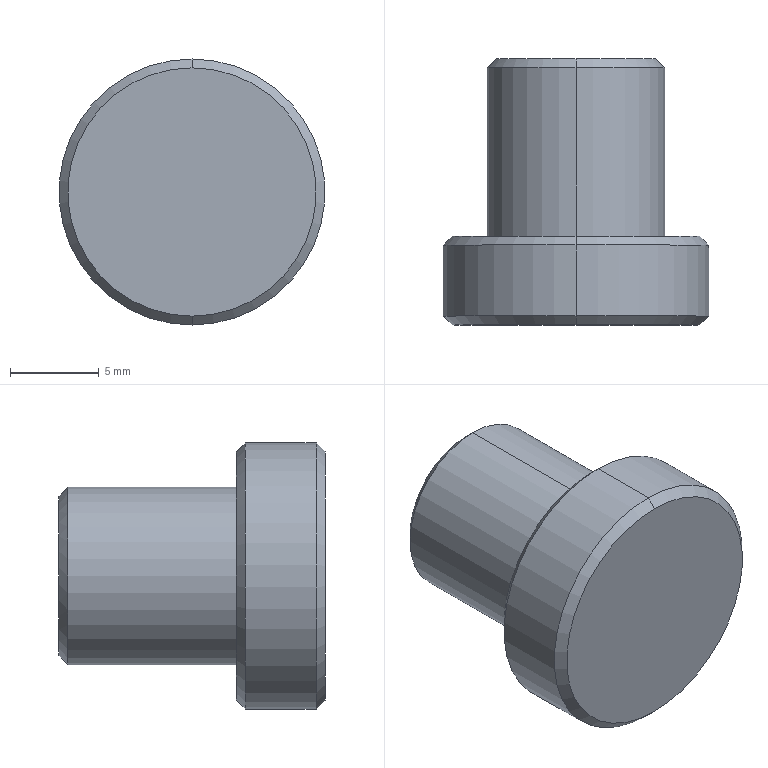Part | SolidWorks | features Chamfer 1, Revolution 1 | 1 solid | 13 faces | box 15 x 15 x 15 mm | volume 1654 mm3 | cone 6 | cylinder 4 | plane 3 | commonest cylinder face diameters 10 x2 15 x2
STEP:
#1=CARTESIAN_POINT('',(0.,15.,4.5));
#2=VERTEX_POINT('',#1);
#3=CARTESIAN_POINT('',(0.,15.,-4.5));
#4=VERTEX_POINT('',#3);
#5=CARTESIAN_POINT('',(0.,15.,0.));
#6=DIRECTION('',(0.,1.,0.));
#7=DIRECTION('',(0.,0.,1.));
#8=AXIS2_PLACEMENT_3D('',#5,#6,#7);
#9=CIRCLE('',#8,4.5);
#10=EDGE_CURVE('',#2,#4,#9,.T.);
#11=ORIENTED_EDGE('',*,*,#10,.F.);
#12=CARTESIAN_POINT('',(0.,14.5,5.));
#13=VERTEX_POINT('',#12);
#14=CARTESIAN_POINT('',(0.,14.5,5.));
#15=DIRECTION('',(0.,-0.7071,0.7071));
#16=VECTOR('',#15,1000.);
#17=LINE('',#14,#16);
#18=EDGE_CURVE('',#2,#13,#17,.T.);
#19=ORIENTED_EDGE('',*,*,#18,.T.);
#20=CARTESIAN_POINT('',(0.,14.5,-5.));
#21=VERTEX_POINT('',#20);
#22=CARTESIAN_POINT('',(0.,14.5,0.));
#23=DIRECTION('',(0.,-1.,0.));
#24=DIRECTION('',(0.,0.,1.));
#25=AXIS2_PLACEMENT_3D('',#22,#23,#24);
#26=CIRCLE('',#25,5.);
#27=EDGE_CURVE('',#21,#13,#26,.T.);
#28=ORIENTED_EDGE('',*,*,#27,.F.);
#29=CARTESIAN_POINT('',(0.,14.5,-5.));
#30=DIRECTION('',(0.,-0.7071,-0.7071));
#31=VECTOR('',#30,1000.);
#32=LINE('',#29,#31);
#33=EDGE_CURVE('',#4,#21,#32,.T.);
#34=ORIENTED_EDGE('',*,*,#33,.F.);
#35=EDGE_LOOP('',(#11,#19,#28,#34));
#36=FACE_OUTER_BOUND('',#35,.T.);
#37=CARTESIAN_POINT('',(0.,14.5,0.));
#38=DIRECTION('',(0.,-1.,0.));
#39=DIRECTION('',(0.,0.,-1.));
#40=AXIS2_PLACEMENT_3D('',#37,#38,#39);
#41=CONICAL_SURFACE('',#40,5.,0.7854);
#42=ADVANCED_FACE('',(#36),#41,.T.);
#43=CARTESIAN_POINT('',(0.,5.,7.));
#44=VERTEX_POINT('',#43);
#45=CARTESIAN_POINT('',(0.,5.,-7.));
#46=VERTEX_POINT('',#45);
#47=CARTESIAN_POINT('',(0.,5.,0.));
#48=DIRECTION('',(0.,1.,0.));
#49=DIRECTION('',(0.,0.,1.));
#50=AXIS2_PLACEMENT_3D('',#47,#48,#49);
#51=CIRCLE('',#50,7.);
#52=EDGE_CURVE('',#44,#46,#51,.T.);
#53=ORIENTED_EDGE('',*,*,#52,.F.);
#54=CARTESIAN_POINT('',(0.,4.5,7.5));
#55=VERTEX_POINT('',#54);
#56=CARTESIAN_POINT('',(0.,4.5,7.5));
#57=DIRECTION('',(0.,-0.7071,0.7071));
#58=VECTOR('',#57,1000.);
#59=LINE('',#56,#58);
#60=EDGE_CURVE('',#44,#55,#59,.T.);
#61=ORIENTED_EDGE('',*,*,#60,.T.);
#62=CARTESIAN_POINT('',(0.,4.5,-7.5));
#63=VERTEX_POINT('',#62);
#64=CARTESIAN_POINT('',(0.,4.5,0.));
#65=DIRECTION('',(0.,-1.,0.));
#66=DIRECTION('',(0.,0.,1.));
#67=AXIS2_PLACEMENT_3D('',#64,#65,#66);
#68=CIRCLE('',#67,7.5);
#69=EDGE_CURVE('',#63,#55,#68,.T.);
#70=ORIENTED_EDGE('',*,*,#69,.F.);
#71=CARTESIAN_POINT('',(0.,4.5,-7.5));
#72=DIRECTION('',(0.,-0.7071,-0.7071));
#73=VECTOR('',#72,1000.);
#74=LINE('',#71,#73);
#75=EDGE_CURVE('',#46,#63,#74,.T.);
#76=ORIENTED_EDGE('',*,*,#75,.F.);
#77=EDGE_LOOP('',(#53,#61,#70,#76));
#78=FACE_OUTER_BOUND('',#77,.T.);
#79=CARTESIAN_POINT('',(0.,4.5,0.));
#80=DIRECTION('',(0.,-1.,0.));
#81=DIRECTION('',(0.,0.,-1.));
#82=AXIS2_PLACEMENT_3D('',#79,#80,#81);
#83=CONICAL_SURFACE('',#82,7.5,0.7854);
#84=ADVANCED_FACE('',(#78),#83,.T.);
#85=CARTESIAN_POINT('',(0.,0.,-7.));
#86=VERTEX_POINT('',#85);
#87=CARTESIAN_POINT('',(0.,0.,7.));
#88=VERTEX_POINT('',#87);
#89=CARTESIAN_POINT('',(0.,0.,0.));
#90=DIRECTION('',(0.,-1.,0.));
#91=DIRECTION('',(0.,0.,-1.));
#92=AXIS2_PLACEMENT_3D('',#89,#90,#91);
#93=CIRCLE('',#92,7.);
#94=EDGE_CURVE('',#86,#88,#93,.T.);
#95=ORIENTED_EDGE('',*,*,#94,.F.);
#96=CARTESIAN_POINT('',(0.,0.5,-7.5));
#97=VERTEX_POINT('',#96);
#98=CARTESIAN_POINT('',(0.,0.,-7.));
#99=DIRECTION('',(0.,0.7071,-0.7071));
#100=VECTOR('',#99,1000.);
#101=LINE('',#98,#100);
#102=EDGE_CURVE('',#86,#97,#101,.T.);
#103=ORIENTED_EDGE('',*,*,#102,.T.);
#104=CARTESIAN_POINT('',(0.,0.5,7.5));
#105=VERTEX_POINT('',#104);
#106=CARTESIAN_POINT('',(0.,0.5,0.));
#107=DIRECTION('',(0.,1.,0.));
#108=DIRECTION('',(0.,0.,-1.));
#109=AXIS2_PLACEMENT_3D('',#106,#107,#108);
#110=CIRCLE('',#109,7.5);
#111=EDGE_CURVE('',#105,#97,#110,.T.);
#112=ORIENTED_EDGE('',*,*,#111,.F.);
#113=CARTESIAN_POINT('',(0.,0.,7.));
#114=DIRECTION('',(0.,0.7071,0.7071));
#115=VECTOR('',#114,1000.);
#116=LINE('',#113,#115);
#117=EDGE_CURVE('',#88,#105,#116,.T.);
#118=ORIENTED_EDGE('',*,*,#117,.F.);
#119=EDGE_LOOP('',(#95,#103,#112,#118));
#120=FACE_OUTER_BOUND('',#119,.T.);
#121=CARTESIAN_POINT('',(0.,0.,0.));
#122=DIRECTION('',(0.,1.,0.));
#123=DIRECTION('',(0.,0.,1.));
#124=AXIS2_PLACEMENT_3D('',#121,#122,#123);
#125=CONICAL_SURFACE('',#124,7.,0.7854);
#126=ADVANCED_FACE('',(#120),#125,.T.);
#127=ORIENTED_EDGE('',*,*,#69,.T.);
#128=CARTESIAN_POINT('',(0.,0.,7.5));
#129=DIRECTION('',(0.,-1.,0.));
#130=VECTOR('',#129,1000.);
#131=LINE('',#128,#130);
#132=EDGE_CURVE('',#55,#105,#131,.T.);
#133=ORIENTED_EDGE('',*,*,#132,.T.);
#134=ORIENTED_EDGE('',*,*,#111,.T.);
#135=CARTESIAN_POINT('',(0.,0.,-7.5));
#136=DIRECTION('',(0.,-1.,0.));
#137=VECTOR('',#136,1000.);
#138=LINE('',#135,#137);
#139=EDGE_CURVE('',#63,#97,#138,.T.);
#140=ORIENTED_EDGE('',*,*,#139,.F.);
#141=EDGE_LOOP('',(#127,#133,#134,#140));
#142=FACE_OUTER_BOUND('',#141,.T.);
#143=CARTESIAN_POINT('',(0.,0.,0.));
#144=DIRECTION('',(0.,-1.,0.));
#145=DIRECTION('',(0.,0.,-1.));
#146=AXIS2_PLACEMENT_3D('',#143,#144,#145);
#147=CYLINDRICAL_SURFACE('',#146,7.5);
#148=ADVANCED_FACE('',(#142),#147,.T.);
#149=ORIENTED_EDGE('',*,*,#27,.T.);
#150=CARTESIAN_POINT('',(0.,5.,5.));
#151=VERTEX_POINT('',#150);
#152=CARTESIAN_POINT('',(0.,0.,5.));
#153=DIRECTION('',(0.,-1.,0.));
#154=VECTOR('',#153,1000.);
#155=LINE('',#152,#154);
#156=EDGE_CURVE('',#13,#151,#155,.T.);
#157=ORIENTED_EDGE('',*,*,#156,.T.);
#158=CARTESIAN_POINT('',(0.,5.,-5.));
#159=VERTEX_POINT('',#158);
#160=CARTESIAN_POINT('',(0.,5.,0.));
#161=DIRECTION('',(0.,-1.,0.));
#162=DIRECTION('',(0.,0.,-1.));
#163=AXIS2_PLACEMENT_3D('',#160,#161,#162);
#164=CIRCLE('',#163,5.);
#165=EDGE_CURVE('',#159,#151,#164,.T.);
#166=ORIENTED_EDGE('',*,*,#165,.F.);
#167=CARTESIAN_POINT('',(0.,0.,-5.));
#168=DIRECTION('',(0.,-1.,0.));
#169=VECTOR('',#168,1000.);
#170=LINE('',#167,#169);
#171=EDGE_CURVE('',#21,#159,#170,.T.);
#172=ORIENTED_EDGE('',*,*,#171,.F.);
#173=EDGE_LOOP('',(#149,#157,#166,#172));
#174=FACE_OUTER_BOUND('',#173,.T.);
#175=CARTESIAN_POINT('',(0.,0.,0.));
#176=DIRECTION('',(0.,-1.,0.));
#177=DIRECTION('',(0.,0.,-1.));
#178=AXIS2_PLACEMENT_3D('',#175,#176,#177);
#179=CYLINDRICAL_SURFACE('',#178,5.);
#180=ADVANCED_FACE('',(#174),#179,.T.);
#181=CARTESIAN_POINT('',(0.,15.,0.));
#182=DIRECTION('',(0.,1.,0.));
#183=DIRECTION('',(0.,0.,1.));
#184=AXIS2_PLACEMENT_3D('',#181,#182,#183);
#185=CIRCLE('',#184,4.5);
#186=EDGE_CURVE('',#4,#2,#185,.T.);
#187=ORIENTED_EDGE('',*,*,#186,.T.);
#188=ORIENTED_EDGE('',*,*,#10,.T.);
#189=EDGE_LOOP('',(#187,#188));
#190=FACE_OUTER_BOUND('',#189,.T.);
#191=CARTESIAN_POINT('',(0.,15.,0.));
#192=DIRECTION('',(0.,1.,0.));
#193=DIRECTION('',(0.,0.,1.));
#194=AXIS2_PLACEMENT_3D('',#191,#192,#193);
#195=PLANE('',#194);
#196=ADVANCED_FACE('',(#190),#195,.T.);
#197=ORIENTED_EDGE('',*,*,#156,.F.);
#198=CARTESIAN_POINT('',(0.,14.5,0.));
#199=DIRECTION('',(0.,-1.,0.));
#200=DIRECTION('',(0.,0.,1.));
#201=AXIS2_PLACEMENT_3D('',#198,#199,#200);
#202=CIRCLE('',#201,5.);
#203=EDGE_CURVE('',#13,#21,#202,.T.);
#204=ORIENTED_EDGE('',*,*,#203,.T.);
#205=ORIENTED_EDGE('',*,*,#171,.T.);
#206=CARTESIAN_POINT('',(0.,5.,0.));
#207=DIRECTION('',(0.,-1.,0.));
#208=DIRECTION('',(0.,0.,-1.));
#209=AXIS2_PLACEMENT_3D('',#206,#207,#208);
#210=CIRCLE('',#209,5.);
#211=EDGE_CURVE('',#151,#159,#210,.T.);
#212=ORIENTED_EDGE('',*,*,#211,.F.);
#213=EDGE_LOOP('',(#197,#204,#205,#212));
#214=FACE_OUTER_BOUND('',#213,.T.);
#215=CARTESIAN_POINT('',(0.,0.,0.));
#216=DIRECTION('',(0.,-1.,0.));
#217=DIRECTION('',(0.,0.,-1.));
#218=AXIS2_PLACEMENT_3D('',#215,#216,#217);
#219=CYLINDRICAL_SURFACE('',#218,5.);
#220=ADVANCED_FACE('',(#214),#219,.T.);
#221=CARTESIAN_POINT('',(0.,5.,0.));
#222=DIRECTION('',(0.,1.,0.));
#223=DIRECTION('',(0.,0.,1.));
#224=AXIS2_PLACEMENT_3D('',#221,#222,#223);
#225=CIRCLE('',#224,7.);
#226=EDGE_CURVE('',#46,#44,#225,.T.);
#227=ORIENTED_EDGE('',*,*,#226,.T.);
#228=ORIENTED_EDGE('',*,*,#52,.T.);
#229=EDGE_LOOP('',(#227,#228));
#230=FACE_OUTER_BOUND('',#229,.T.);
#231=ORIENTED_EDGE('',*,*,#165,.T.);
#232=ORIENTED_EDGE('',*,*,#211,.T.);
#233=EDGE_LOOP('',(#231,#232));
#234=FACE_BOUND('',#233,.T.);
#235=CARTESIAN_POINT('',(0.,5.,-5.));
#236=DIRECTION('',(0.,1.,0.));
#237=DIRECTION('',(0.,0.,1.));
#238=AXIS2_PLACEMENT_3D('',#235,#236,#237);
#239=PLANE('',#238);
#240=ADVANCED_FACE('',(#230,#234),#239,.T.);
#241=ORIENTED_EDGE('',*,*,#132,.F.);
#242=CARTESIAN_POINT('',(0.,4.5,0.));
#243=DIRECTION('',(0.,-1.,0.));
#244=DIRECTION('',(0.,0.,1.));
#245=AXIS2_PLACEMENT_3D('',#242,#243,#244);
#246=CIRCLE('',#245,7.5);
#247=EDGE_CURVE('',#55,#63,#246,.T.);
#248=ORIENTED_EDGE('',*,*,#247,.T.);
#249=ORIENTED_EDGE('',*,*,#139,.T.);
#250=CARTESIAN_POINT('',(0.,0.5,0.));
#251=DIRECTION('',(0.,1.,0.));
#252=DIRECTION('',(0.,0.,-1.));
#253=AXIS2_PLACEMENT_3D('',#250,#251,#252);
#254=CIRCLE('',#253,7.5);
#255=EDGE_CURVE('',#97,#105,#254,.T.);
#256=ORIENTED_EDGE('',*,*,#255,.T.);
#257=EDGE_LOOP('',(#241,#248,#249,#256));
#258=FACE_OUTER_BOUND('',#257,.T.);
#259=CARTESIAN_POINT('',(0.,0.,0.));
#260=DIRECTION('',(0.,-1.,0.));
#261=DIRECTION('',(0.,0.,-1.));
#262=AXIS2_PLACEMENT_3D('',#259,#260,#261);
#263=CYLINDRICAL_SURFACE('',#262,7.5);
#264=ADVANCED_FACE('',(#258),#263,.T.);
#265=CARTESIAN_POINT('',(0.,0.,0.));
#266=DIRECTION('',(0.,-1.,0.));
#267=DIRECTION('',(0.,0.,-1.));
#268=AXIS2_PLACEMENT_3D('',#265,#266,#267);
#269=CIRCLE('',#268,7.);
#270=EDGE_CURVE('',#88,#86,#269,.T.);
#271=ORIENTED_EDGE('',*,*,#270,.T.);
#272=ORIENTED_EDGE('',*,*,#94,.T.);
#273=EDGE_LOOP('',(#271,#272));
#274=FACE_OUTER_BOUND('',#273,.T.);
#275=CARTESIAN_POINT('',(0.,0.,-7.5));
#276=DIRECTION('',(0.,-1.,0.));
#277=DIRECTION('',(0.,0.,-1.));
#278=AXIS2_PLACEMENT_3D('',#275,#276,#277);
#279=PLANE('',#278);
#280=ADVANCED_FACE('',(#274),#279,.T.);
#281=ORIENTED_EDGE('',*,*,#102,.F.);
#282=ORIENTED_EDGE('',*,*,#270,.F.);
#283=ORIENTED_EDGE('',*,*,#117,.T.);
#284=ORIENTED_EDGE('',*,*,#255,.F.);
#285=EDGE_LOOP('',(#281,#282,#283,#284));
#286=FACE_OUTER_BOUND('',#285,.T.);
#287=CARTESIAN_POINT('',(0.,0.,0.));
#288=DIRECTION('',(0.,1.,0.));
#289=DIRECTION('',(0.,0.,1.));
#290=AXIS2_PLACEMENT_3D('',#287,#288,#289);
#291=CONICAL_SURFACE('',#290,7.,0.7854);
#292=ADVANCED_FACE('',(#286),#291,.T.);
#293=ORIENTED_EDGE('',*,*,#60,.F.);
#294=ORIENTED_EDGE('',*,*,#226,.F.);
#295=ORIENTED_EDGE('',*,*,#75,.T.);
#296=ORIENTED_EDGE('',*,*,#247,.F.);
#297=EDGE_LOOP('',(#293,#294,#295,#296));
#298=FACE_OUTER_BOUND('',#297,.T.);
#299=CARTESIAN_POINT('',(0.,4.5,0.));
#300=DIRECTION('',(0.,-1.,0.));
#301=DIRECTION('',(0.,0.,-1.));
#302=AXIS2_PLACEMENT_3D('',#299,#300,#301);
#303=CONICAL_SURFACE('',#302,7.5,0.7854);
#304=ADVANCED_FACE('',(#298),#303,.T.);
#305=ORIENTED_EDGE('',*,*,#18,.F.);
#306=ORIENTED_EDGE('',*,*,#186,.F.);
#307=ORIENTED_EDGE('',*,*,#33,.T.);
#308=ORIENTED_EDGE('',*,*,#203,.F.);
#309=EDGE_LOOP('',(#305,#306,#307,#308));
#310=FACE_OUTER_BOUND('',#309,.T.);
#311=CARTESIAN_POINT('',(0.,14.5,0.));
#312=DIRECTION('',(0.,-1.,0.));
#313=DIRECTION('',(0.,0.,-1.));
#314=AXIS2_PLACEMENT_3D('',#311,#312,#313);
#315=CONICAL_SURFACE('',#314,5.,0.7854);
#316=ADVANCED_FACE('',(#310),#315,.T.);
#317=CLOSED_SHELL('',(#42,#84,#126,#148,#180,#196,#220,#240,#264,#280,#292,#304,#316));
#318=MANIFOLD_SOLID_BREP('',#317);
#319=CARTESIAN_POINT('',(0.,0.,0.));
#320=DIRECTION('',(0.,0.,1.));
#321=DIRECTION('',(1.,0.,0.));
#322=AXIS2_PLACEMENT_3D('',#319,#320,#321);
#323=(LENGTH_UNIT()NAMED_UNIT(*)SI_UNIT(.MILLI.,.METRE.));
#324=UNCERTAINTY_MEASURE_WITH_UNIT(LENGTH_MEASURE(0.00001),#323,'','');
#325=(NAMED_UNIT(*)PLANE_ANGLE_UNIT()SI_UNIT($,.RADIAN.));
#326=(NAMED_UNIT(*)SI_UNIT($,.STERADIAN.)SOLID_ANGLE_UNIT());
#327=(GEOMETRIC_REPRESENTATION_CONTEXT(3)GLOBAL_UNCERTAINTY_ASSIGNED_CONTEXT((#324))GLOBAL_UNIT_ASSIGNED_CONTEXT((#323,#325,#326))REPRESENTATION_CONTEXT('',''));
#328=ADVANCED_BREP_SHAPE_REPRESENTATION('',(#318,#322),#327);